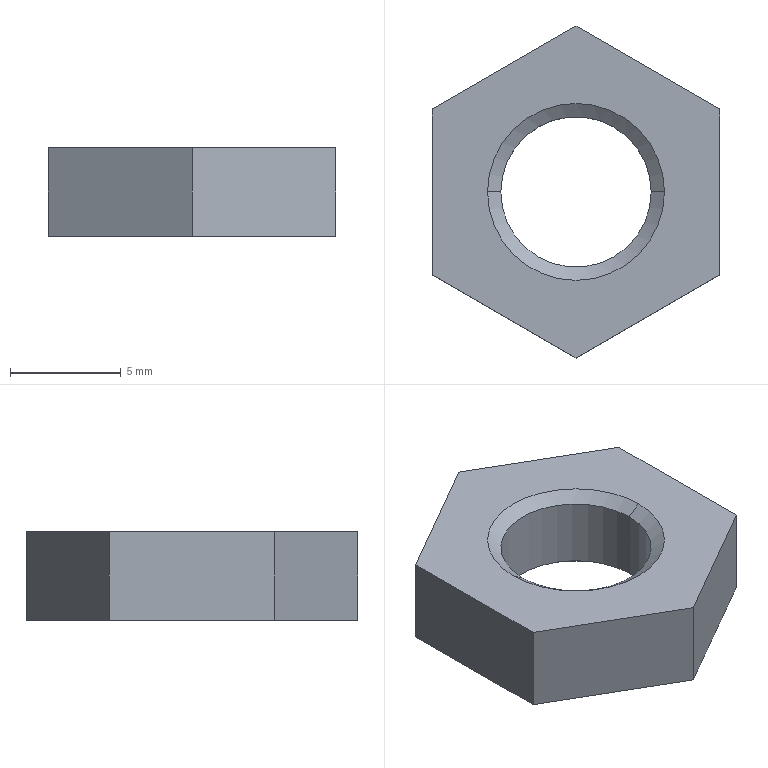Part | STEP file | hex thin nut gradeb_iso(Hexagon Nut ISO - 4036 - M8 - N) | 1 solid | 16 faces | box 13 x 15.011 x 4 mm | volume 434.11 mm3 | plane 8 | cylinder 4 | cone 4 | commonest cylinder face diameters 6.8 x2 8 x2
STEP:
#1=CARTESIAN_POINT('',(0.,0.,0.));
#2=DIRECTION('',(0.,0.,1.));
#3=DIRECTION('',(1.,0.,0.));
#4=AXIS2_PLACEMENT_3D('',#1,#2,#3);
#5=CARTESIAN_POINT('',(4.,0.,-4.));
#6=VERTEX_POINT('',#5);
#7=CARTESIAN_POINT('',(4.,0.,-3.975));
#8=VERTEX_POINT('',#7);
#9=CARTESIAN_POINT('',(4.,0.,-25.038));
#10=DIRECTION('',(0.,0.,1.));
#11=VECTOR('',#10,1.);
#12=LINE('',#9,#11);
#13=CARTESIAN_POINT('',(0.,0.,-25.038));
#14=DIRECTION('',(0.,0.,1.));
#15=DIRECTION('',(1.,0.,0.));
#16=AXIS2_PLACEMENT_3D('',#13,#14,#15);
#17=CYLINDRICAL_SURFACE('',#16,4.);
#18=CARTESIAN_POINT('',(6.283,0.));
#19=DIRECTION('',(0.,1.));
#20=VECTOR('',#19,1.);
#21=LINE('',#18,#20);
#22=(GEOMETRIC_REPRESENTATION_CONTEXT(2)PARAMETRIC_REPRESENTATION_CONTEXT()REPRESENTATION_CONTEXT('',''));
#23=DEFINITIONAL_REPRESENTATION('',(#21),#22);
#24=PCURVE('',#17,#23);
#25=CARTESIAN_POINT('',(0.,0.,-25.038));
#26=DIRECTION('',(0.,0.,1.));
#27=DIRECTION('',(1.,0.,0.));
#28=AXIS2_PLACEMENT_3D('',#25,#26,#27);
#29=CYLINDRICAL_SURFACE('',#28,4.);
#30=CARTESIAN_POINT('',(0.,0.));
#31=DIRECTION('',(0.,1.));
#32=VECTOR('',#31,1.);
#33=LINE('',#30,#32);
#34=(GEOMETRIC_REPRESENTATION_CONTEXT(2)PARAMETRIC_REPRESENTATION_CONTEXT()REPRESENTATION_CONTEXT('',''));
#35=DEFINITIONAL_REPRESENTATION('',(#33),#34);
#36=PCURVE('',#29,#35);
#37=SURFACE_CURVE('',#12,(#24,#36),.PCURVE_S1.);
#38=EDGE_CURVE('',#6,#8,#37,.T.);
#39=ORIENTED_EDGE('',*,*,#38,.T.);
#40=CARTESIAN_POINT('',(-4.,0.,-3.975));
#41=VERTEX_POINT('',#40);
#42=CARTESIAN_POINT('',(0.,0.,-3.975));
#43=DIRECTION('',(0.,0.,1.));
#44=DIRECTION('',(1.,0.,0.));
#45=AXIS2_PLACEMENT_3D('',#42,#43,#44);
#46=CIRCLE('',#45,4.);
#47=CARTESIAN_POINT('',(0.,21.063));
#48=DIRECTION('',(1.,0.));
#49=VECTOR('',#48,1.);
#50=LINE('',#47,#49);
#51=(GEOMETRIC_REPRESENTATION_CONTEXT(2)PARAMETRIC_REPRESENTATION_CONTEXT()REPRESENTATION_CONTEXT('',''));
#52=DEFINITIONAL_REPRESENTATION('',(#50),#51);
#53=PCURVE('',#17,#52);
#54=CARTESIAN_POINT('',(0.,0.,-3.975));
#55=DIRECTION('',(0.,0.,-1.));
#56=DIRECTION('',(-1.,0.,0.));
#57=AXIS2_PLACEMENT_3D('',#54,#55,#56);
#58=CONICAL_SURFACE('',#57,4.,0.9599);
#59=CARTESIAN_POINT('',(9.425,0.));
#60=DIRECTION('',(-1.,0.));
#61=VECTOR('',#60,1.);
#62=LINE('',#59,#61);
#63=(GEOMETRIC_REPRESENTATION_CONTEXT(2)PARAMETRIC_REPRESENTATION_CONTEXT()REPRESENTATION_CONTEXT('',''));
#64=DEFINITIONAL_REPRESENTATION('',(#62),#63);
#65=PCURVE('',#58,#64);
#66=SURFACE_CURVE('',#46,(#53,#65),.PCURVE_S1.);
#67=EDGE_CURVE('',#41,#8,#66,.T.);
#68=ORIENTED_EDGE('',*,*,#67,.F.);
#69=CARTESIAN_POINT('',(-4.,0.,-4.));
#70=VERTEX_POINT('',#69);
#71=CARTESIAN_POINT('',(-4.,0.,-25.038));
#72=DIRECTION('',(0.,0.,1.));
#73=VECTOR('',#72,1.);
#74=LINE('',#71,#73);
#75=CARTESIAN_POINT('',(3.142,0.));
#76=DIRECTION('',(0.,1.));
#77=VECTOR('',#76,1.);
#78=LINE('',#75,#77);
#79=(GEOMETRIC_REPRESENTATION_CONTEXT(2)PARAMETRIC_REPRESENTATION_CONTEXT()REPRESENTATION_CONTEXT('',''));
#80=DEFINITIONAL_REPRESENTATION('',(#78),#79);
#81=PCURVE('',#17,#80);
#82=CARTESIAN_POINT('',(3.142,0.));
#83=DIRECTION('',(0.,1.));
#84=VECTOR('',#83,1.);
#85=LINE('',#82,#84);
#86=(GEOMETRIC_REPRESENTATION_CONTEXT(2)PARAMETRIC_REPRESENTATION_CONTEXT()REPRESENTATION_CONTEXT('',''));
#87=DEFINITIONAL_REPRESENTATION('',(#85),#86);
#88=PCURVE('',#29,#87);
#89=SURFACE_CURVE('',#74,(#81,#88),.PCURVE_S1.);
#90=EDGE_CURVE('',#70,#41,#89,.T.);
#91=ORIENTED_EDGE('',*,*,#90,.F.);
#92=CARTESIAN_POINT('',(0.,0.,-4.));
#93=DIRECTION('',(0.,0.,1.));
#94=DIRECTION('',(-1.,0.,0.));
#95=AXIS2_PLACEMENT_3D('',#92,#93,#94);
#96=CIRCLE('',#95,4.);
#97=CARTESIAN_POINT('',(3.142,21.038));
#98=DIRECTION('',(1.,0.));
#99=VECTOR('',#98,1.);
#100=LINE('',#97,#99);
#101=(GEOMETRIC_REPRESENTATION_CONTEXT(2)PARAMETRIC_REPRESENTATION_CONTEXT()REPRESENTATION_CONTEXT('',''));
#102=DEFINITIONAL_REPRESENTATION('',(#100),#101);
#103=PCURVE('',#17,#102);
#104=CARTESIAN_POINT('',(0.,7.506,-4.));
#105=DIRECTION('',(0.,0.,-1.));
#106=DIRECTION('',(-1.,0.,0.));
#107=AXIS2_PLACEMENT_3D('',#104,#105,#106);
#108=PLANE('',#107);
#109=CARTESIAN_POINT('',(4.,-7.506));
#110=CARTESIAN_POINT('',(4.,-14.434));
#111=CARTESIAN_POINT('',(-2.,-10.97));
#112=CARTESIAN_POINT('',(-8.,-7.506));
#113=CARTESIAN_POINT('',(-2.,-4.041));
#114=CARTESIAN_POINT('',(4.,-0.5774));
#115=CARTESIAN_POINT('',(4.,-7.506));
#116=(BOUNDED_CURVE()B_SPLINE_CURVE(2,(#109,#110,#111,#112,#113,#114,#115),.UNSPECIFIED.,.T.,.F.)B_SPLINE_CURVE_WITH_KNOTS((1,2,2,2,2,1),(-2.094,0.,2.094,4.189,6.283,8.378),.UNSPECIFIED.)CURVE()GEOMETRIC_REPRESENTATION_ITEM()RATIONAL_B_SPLINE_CURVE((1.,0.5,1.,0.5,1.,0.5,1.))REPRESENTATION_ITEM(''));
#117=(GEOMETRIC_REPRESENTATION_CONTEXT(2)PARAMETRIC_REPRESENTATION_CONTEXT()REPRESENTATION_CONTEXT('',''));
#118=DEFINITIONAL_REPRESENTATION('',(#116),#117);
#119=PCURVE('',#108,#118);
#120=SURFACE_CURVE('',#96,(#103,#119),.PCURVE_S1.);
#121=EDGE_CURVE('',#70,#6,#120,.T.);
#122=ORIENTED_EDGE('',*,*,#121,.T.);
#123=EDGE_LOOP('',(#39,#68,#91,#122));
#124=FACE_BOUND('',#123,.F.);
#125=ADVANCED_FACE('',(#124),#17,.F.);
#126=CARTESIAN_POINT('',(-3.4,0.,-3.554));
#127=VERTEX_POINT('',#126);
#128=CARTESIAN_POINT('',(-4.,0.,-3.975));
#129=DIRECTION('',(-0.8192,0.,-0.5736));
#130=VECTOR('',#129,1.);
#131=LINE('',#128,#130);
#132=CARTESIAN_POINT('',(6.283,0.));
#133=DIRECTION('',(0.,1.));
#134=VECTOR('',#133,1.);
#135=LINE('',#132,#134);
#136=(GEOMETRIC_REPRESENTATION_CONTEXT(2)PARAMETRIC_REPRESENTATION_CONTEXT()REPRESENTATION_CONTEXT('',''));
#137=DEFINITIONAL_REPRESENTATION('',(#135),#136);
#138=PCURVE('',#58,#137);
#139=CARTESIAN_POINT('',(0.,0.,-3.975));
#140=DIRECTION('',(0.,0.,-1.));
#141=DIRECTION('',(-1.,0.,0.));
#142=AXIS2_PLACEMENT_3D('',#139,#140,#141);
#143=CONICAL_SURFACE('',#142,4.,0.9599);
#144=CARTESIAN_POINT('',(0.,0.));
#145=DIRECTION('',(0.,1.));
#146=VECTOR('',#145,1.);
#147=LINE('',#144,#146);
#148=(GEOMETRIC_REPRESENTATION_CONTEXT(2)PARAMETRIC_REPRESENTATION_CONTEXT()REPRESENTATION_CONTEXT('',''));
#149=DEFINITIONAL_REPRESENTATION('',(#147),#148);
#150=PCURVE('',#143,#149);
#151=SURFACE_CURVE('',#131,(#138,#150),.PCURVE_S1.);
#152=EDGE_CURVE('',#127,#41,#151,.T.);
#153=ORIENTED_EDGE('',*,*,#152,.T.);
#154=ORIENTED_EDGE('',*,*,#67,.T.);
#155=CARTESIAN_POINT('',(3.4,0.,-3.554));
#156=VERTEX_POINT('',#155);
#157=CARTESIAN_POINT('',(4.,0.,-3.975));
#158=DIRECTION('',(0.8192,0.,-0.5736));
#159=VECTOR('',#158,1.);
#160=LINE('',#157,#159);
#161=CARTESIAN_POINT('',(3.142,0.));
#162=DIRECTION('',(0.,1.));
#163=VECTOR('',#162,1.);
#164=LINE('',#161,#163);
#165=(GEOMETRIC_REPRESENTATION_CONTEXT(2)PARAMETRIC_REPRESENTATION_CONTEXT()REPRESENTATION_CONTEXT('',''));
#166=DEFINITIONAL_REPRESENTATION('',(#164),#165);
#167=PCURVE('',#58,#166);
#168=CARTESIAN_POINT('',(3.142,0.));
#169=DIRECTION('',(0.,1.));
#170=VECTOR('',#169,1.);
#171=LINE('',#168,#170);
#172=(GEOMETRIC_REPRESENTATION_CONTEXT(2)PARAMETRIC_REPRESENTATION_CONTEXT()REPRESENTATION_CONTEXT('',''));
#173=DEFINITIONAL_REPRESENTATION('',(#171),#172);
#174=PCURVE('',#143,#173);
#175=SURFACE_CURVE('',#160,(#167,#174),.PCURVE_S1.);
#176=EDGE_CURVE('',#156,#8,#175,.T.);
#177=ORIENTED_EDGE('',*,*,#176,.F.);
#178=CARTESIAN_POINT('',(0.,0.,-3.554));
#179=DIRECTION('',(0.,0.,1.));
#180=DIRECTION('',(-1.,0.,0.));
#181=AXIS2_PLACEMENT_3D('',#178,#179,#180);
#182=CIRCLE('',#181,3.4);
#183=CARTESIAN_POINT('',(6.283,-0.4201));
#184=DIRECTION('',(-1.,0.));
#185=VECTOR('',#184,1.);
#186=LINE('',#183,#185);
#187=(GEOMETRIC_REPRESENTATION_CONTEXT(2)PARAMETRIC_REPRESENTATION_CONTEXT()REPRESENTATION_CONTEXT('',''));
#188=DEFINITIONAL_REPRESENTATION('',(#186),#187);
#189=PCURVE('',#58,#188);
#190=CARTESIAN_POINT('',(0.,0.,-4.));
#191=DIRECTION('',(0.,0.,1.));
#192=DIRECTION('',(1.,0.,0.));
#193=AXIS2_PLACEMENT_3D('',#190,#191,#192);
#194=CYLINDRICAL_SURFACE('',#193,3.4);
#195=CARTESIAN_POINT('',(3.142,0.4455));
#196=DIRECTION('',(1.,0.));
#197=VECTOR('',#196,1.);
#198=LINE('',#195,#197);
#199=(GEOMETRIC_REPRESENTATION_CONTEXT(2)PARAMETRIC_REPRESENTATION_CONTEXT()REPRESENTATION_CONTEXT('',''));
#200=DEFINITIONAL_REPRESENTATION('',(#198),#199);
#201=PCURVE('',#194,#200);
#202=SURFACE_CURVE('',#182,(#189,#201),.PCURVE_S1.);
#203=EDGE_CURVE('',#127,#156,#202,.T.);
#204=ORIENTED_EDGE('',*,*,#203,.F.);
#205=EDGE_LOOP('',(#153,#154,#177,#204));
#206=FACE_BOUND('',#205,.F.);
#207=ADVANCED_FACE('',(#206),#58,.F.);
#208=CARTESIAN_POINT('',(3.4,0.,-0.4201));
#209=VERTEX_POINT('',#208);
#210=CARTESIAN_POINT('',(4.,0.,0.));
#211=VERTEX_POINT('',#210);
#212=CARTESIAN_POINT('',(3.34,0.,-0.4621));
#213=DIRECTION('',(0.8192,0.,0.5736));
#214=VECTOR('',#213,1.);
#215=LINE('',#212,#214);
#216=CARTESIAN_POINT('',(0.,0.,-0.4621));
#217=DIRECTION('',(0.,0.,1.));
#218=DIRECTION('',(1.,0.,0.));
#219=AXIS2_PLACEMENT_3D('',#216,#217,#218);
#220=CONICAL_SURFACE('',#219,3.34,0.9599);
#221=CARTESIAN_POINT('',(6.283,0.));
#222=DIRECTION('',(0.,1.));
#223=VECTOR('',#222,1.);
#224=LINE('',#221,#223);
#225=(GEOMETRIC_REPRESENTATION_CONTEXT(2)PARAMETRIC_REPRESENTATION_CONTEXT()REPRESENTATION_CONTEXT('',''));
#226=DEFINITIONAL_REPRESENTATION('',(#224),#225);
#227=PCURVE('',#220,#226);
#228=CARTESIAN_POINT('',(0.,0.,-0.4621));
#229=DIRECTION('',(0.,0.,1.));
#230=DIRECTION('',(1.,0.,0.));
#231=AXIS2_PLACEMENT_3D('',#228,#229,#230);
#232=CONICAL_SURFACE('',#231,3.34,0.9599);
#233=CARTESIAN_POINT('',(0.,0.));
#234=DIRECTION('',(0.,1.));
#235=VECTOR('',#234,1.);
#236=LINE('',#233,#235);
#237=(GEOMETRIC_REPRESENTATION_CONTEXT(2)PARAMETRIC_REPRESENTATION_CONTEXT()REPRESENTATION_CONTEXT('',''));
#238=DEFINITIONAL_REPRESENTATION('',(#236),#237);
#239=PCURVE('',#232,#238);
#240=SURFACE_CURVE('',#215,(#227,#239),.PCURVE_S1.);
#241=EDGE_CURVE('',#209,#211,#240,.T.);
#242=ORIENTED_EDGE('',*,*,#241,.T.);
#243=CARTESIAN_POINT('',(-4.,0.,0.));
#244=VERTEX_POINT('',#243);
#245=CARTESIAN_POINT('',(0.,0.,0.));
#246=DIRECTION('',(0.,0.,1.));
#247=DIRECTION('',(1.,0.,0.));
#248=AXIS2_PLACEMENT_3D('',#245,#246,#247);
#249=CIRCLE('',#248,4.);
#250=CARTESIAN_POINT('',(0.,0.4621));
#251=DIRECTION('',(1.,0.));
#252=VECTOR('',#251,1.);
#253=LINE('',#250,#252);
#254=(GEOMETRIC_REPRESENTATION_CONTEXT(2)PARAMETRIC_REPRESENTATION_CONTEXT()REPRESENTATION_CONTEXT('',''));
#255=DEFINITIONAL_REPRESENTATION('',(#253),#254);
#256=PCURVE('',#220,#255);
#257=CARTESIAN_POINT('',(0.,7.506,0.));
#258=DIRECTION('',(0.,0.,-1.));
#259=DIRECTION('',(-1.,0.,0.));
#260=AXIS2_PLACEMENT_3D('',#257,#258,#259);
#261=PLANE('',#260);
#262=CARTESIAN_POINT('',(-4.,-7.506));
#263=CARTESIAN_POINT('',(-4.,-0.5774));
#264=CARTESIAN_POINT('',(2.,-4.041));
#265=CARTESIAN_POINT('',(8.,-7.506));
#266=CARTESIAN_POINT('',(2.,-10.97));
#267=CARTESIAN_POINT('',(-4.,-14.434));
#268=CARTESIAN_POINT('',(-4.,-7.506));
#269=(BOUNDED_CURVE()B_SPLINE_CURVE(2,(#262,#263,#264,#265,#266,#267,#268),.UNSPECIFIED.,.T.,.F.)B_SPLINE_CURVE_WITH_KNOTS((1,2,2,2,2,1),(-2.094,0.,2.094,4.189,6.283,8.378),.UNSPECIFIED.)CURVE()GEOMETRIC_REPRESENTATION_ITEM()RATIONAL_B_SPLINE_CURVE((1.,0.5,1.,0.5,1.,0.5,1.))REPRESENTATION_ITEM(''));
#270=(GEOMETRIC_REPRESENTATION_CONTEXT(2)PARAMETRIC_REPRESENTATION_CONTEXT()REPRESENTATION_CONTEXT('',''));
#271=DEFINITIONAL_REPRESENTATION('',(#269),#270);
#272=PCURVE('',#261,#271);
#273=SURFACE_CURVE('',#249,(#256,#272),.PCURVE_S1.);
#274=EDGE_CURVE('',#244,#211,#273,.T.);
#275=ORIENTED_EDGE('',*,*,#274,.F.);
#276=CARTESIAN_POINT('',(-3.4,0.,-0.4201));
#277=VERTEX_POINT('',#276);
#278=CARTESIAN_POINT('',(-3.34,0.,-0.4621));
#279=DIRECTION('',(-0.8192,0.,0.5736));
#280=VECTOR('',#279,1.);
#281=LINE('',#278,#280);
#282=CARTESIAN_POINT('',(3.142,0.));
#283=DIRECTION('',(0.,1.));
#284=VECTOR('',#283,1.);
#285=LINE('',#282,#284);
#286=(GEOMETRIC_REPRESENTATION_CONTEXT(2)PARAMETRIC_REPRESENTATION_CONTEXT()REPRESENTATION_CONTEXT('',''));
#287=DEFINITIONAL_REPRESENTATION('',(#285),#286);
#288=PCURVE('',#220,#287);
#289=CARTESIAN_POINT('',(3.142,0.));
#290=DIRECTION('',(0.,1.));
#291=VECTOR('',#290,1.);
#292=LINE('',#289,#291);
#293=(GEOMETRIC_REPRESENTATION_CONTEXT(2)PARAMETRIC_REPRESENTATION_CONTEXT()REPRESENTATION_CONTEXT('',''));
#294=DEFINITIONAL_REPRESENTATION('',(#292),#293);
#295=PCURVE('',#232,#294);
#296=SURFACE_CURVE('',#281,(#288,#295),.PCURVE_S1.);
#297=EDGE_CURVE('',#277,#244,#296,.T.);
#298=ORIENTED_EDGE('',*,*,#297,.F.);
#299=CARTESIAN_POINT('',(0.,0.,-0.4201));
#300=DIRECTION('',(0.,0.,-1.));
#301=DIRECTION('',(1.,0.,0.));
#302=AXIS2_PLACEMENT_3D('',#299,#300,#301);
#303=CIRCLE('',#302,3.4);
#304=CARTESIAN_POINT('',(6.283,0.04201));
#305=DIRECTION('',(-1.,0.));
#306=VECTOR('',#305,1.);
#307=LINE('',#304,#306);
#308=(GEOMETRIC_REPRESENTATION_CONTEXT(2)PARAMETRIC_REPRESENTATION_CONTEXT()REPRESENTATION_CONTEXT('',''));
#309=DEFINITIONAL_REPRESENTATION('',(#307),#308);
#310=PCURVE('',#220,#309);
#311=CARTESIAN_POINT('',(6.283,3.58));
#312=DIRECTION('',(-1.,0.));
#313=VECTOR('',#312,1.);
#314=LINE('',#311,#313);
#315=(GEOMETRIC_REPRESENTATION_CONTEXT(2)PARAMETRIC_REPRESENTATION_CONTEXT()REPRESENTATION_CONTEXT('',''));
#316=DEFINITIONAL_REPRESENTATION('',(#314),#315);
#317=PCURVE('',#194,#316);
#318=SURFACE_CURVE('',#303,(#310,#317),.PCURVE_S1.);
#319=EDGE_CURVE('',#209,#277,#318,.T.);
#320=ORIENTED_EDGE('',*,*,#319,.F.);
#321=EDGE_LOOP('',(#242,#275,#298,#320));
#322=FACE_BOUND('',#321,.F.);
#323=ADVANCED_FACE('',(#322),#220,.F.);
#324=CARTESIAN_POINT('',(3.4,0.,-4.));
#325=DIRECTION('',(0.,0.,1.));
#326=VECTOR('',#325,1.);
#327=LINE('',#324,#326);
#328=CARTESIAN_POINT('',(6.283,0.));
#329=DIRECTION('',(0.,1.));
#330=VECTOR('',#329,1.);
#331=LINE('',#328,#330);
#332=(GEOMETRIC_REPRESENTATION_CONTEXT(2)PARAMETRIC_REPRESENTATION_CONTEXT()REPRESENTATION_CONTEXT('',''));
#333=DEFINITIONAL_REPRESENTATION('',(#331),#332);
#334=PCURVE('',#194,#333);
#335=CARTESIAN_POINT('',(0.,0.,-4.));
#336=DIRECTION('',(0.,0.,1.));
#337=DIRECTION('',(1.,0.,0.));
#338=AXIS2_PLACEMENT_3D('',#335,#336,#337);
#339=CYLINDRICAL_SURFACE('',#338,3.4);
#340=CARTESIAN_POINT('',(0.,0.));
#341=DIRECTION('',(0.,1.));
#342=VECTOR('',#341,1.);
#343=LINE('',#340,#342);
#344=(GEOMETRIC_REPRESENTATION_CONTEXT(2)PARAMETRIC_REPRESENTATION_CONTEXT()REPRESENTATION_CONTEXT('',''));
#345=DEFINITIONAL_REPRESENTATION('',(#343),#344);
#346=PCURVE('',#339,#345);
#347=SURFACE_CURVE('',#327,(#334,#346),.PCURVE_S1.);
#348=EDGE_CURVE('',#156,#209,#347,.T.);
#349=ORIENTED_EDGE('',*,*,#348,.T.);
#350=ORIENTED_EDGE('',*,*,#319,.T.);
#351=CARTESIAN_POINT('',(-3.4,0.,-4.));
#352=DIRECTION('',(0.,0.,1.));
#353=VECTOR('',#352,1.);
#354=LINE('',#351,#353);
#355=CARTESIAN_POINT('',(3.142,0.));
#356=DIRECTION('',(0.,1.));
#357=VECTOR('',#356,1.);
#358=LINE('',#355,#357);
#359=(GEOMETRIC_REPRESENTATION_CONTEXT(2)PARAMETRIC_REPRESENTATION_CONTEXT()REPRESENTATION_CONTEXT('',''));
#360=DEFINITIONAL_REPRESENTATION('',(#358),#359);
#361=PCURVE('',#194,#360);
#362=CARTESIAN_POINT('',(3.142,0.));
#363=DIRECTION('',(0.,1.));
#364=VECTOR('',#363,1.);
#365=LINE('',#362,#364);
#366=(GEOMETRIC_REPRESENTATION_CONTEXT(2)PARAMETRIC_REPRESENTATION_CONTEXT()REPRESENTATION_CONTEXT('',''));
#367=DEFINITIONAL_REPRESENTATION('',(#365),#366);
#368=PCURVE('',#339,#367);
#369=SURFACE_CURVE('',#354,(#361,#368),.PCURVE_S1.);
#370=EDGE_CURVE('',#127,#277,#369,.T.);
#371=ORIENTED_EDGE('',*,*,#370,.F.);
#372=ORIENTED_EDGE('',*,*,#203,.T.);
#373=EDGE_LOOP('',(#349,#350,#371,#372));
#374=FACE_BOUND('',#373,.F.);
#375=ADVANCED_FACE('',(#374),#194,.F.);
#376=CARTESIAN_POINT('',(0.,0.,-0.4201));
#377=DIRECTION('',(0.,0.,-1.));
#378=DIRECTION('',(1.,0.,0.));
#379=AXIS2_PLACEMENT_3D('',#376,#377,#378);
#380=CIRCLE('',#379,3.4);
#381=CARTESIAN_POINT('',(6.283,3.58));
#382=DIRECTION('',(-1.,0.));
#383=VECTOR('',#382,1.);
#384=LINE('',#381,#383);
#385=(GEOMETRIC_REPRESENTATION_CONTEXT(2)PARAMETRIC_REPRESENTATION_CONTEXT()REPRESENTATION_CONTEXT('',''));
#386=DEFINITIONAL_REPRESENTATION('',(#384),#385);
#387=PCURVE('',#339,#386);
#388=CARTESIAN_POINT('',(6.283,0.04201));
#389=DIRECTION('',(-1.,0.));
#390=VECTOR('',#389,1.);
#391=LINE('',#388,#390);
#392=(GEOMETRIC_REPRESENTATION_CONTEXT(2)PARAMETRIC_REPRESENTATION_CONTEXT()REPRESENTATION_CONTEXT('',''));
#393=DEFINITIONAL_REPRESENTATION('',(#391),#392);
#394=PCURVE('',#232,#393);
#395=SURFACE_CURVE('',#380,(#387,#394),.PCURVE_S1.);
#396=EDGE_CURVE('',#277,#209,#395,.T.);
#397=ORIENTED_EDGE('',*,*,#396,.T.);
#398=ORIENTED_EDGE('',*,*,#348,.F.);
#399=CARTESIAN_POINT('',(0.,0.,-3.554));
#400=DIRECTION('',(0.,0.,1.));
#401=DIRECTION('',(-1.,0.,0.));
#402=AXIS2_PLACEMENT_3D('',#399,#400,#401);
#403=CIRCLE('',#402,3.4);
#404=CARTESIAN_POINT('',(-3.142,0.4455));
#405=DIRECTION('',(1.,0.));
#406=VECTOR('',#405,1.);
#407=LINE('',#404,#406);
#408=(GEOMETRIC_REPRESENTATION_CONTEXT(2)PARAMETRIC_REPRESENTATION_CONTEXT()REPRESENTATION_CONTEXT('',''));
#409=DEFINITIONAL_REPRESENTATION('',(#407),#408);
#410=PCURVE('',#339,#409);
#411=CARTESIAN_POINT('',(6.283,-0.4201));
#412=DIRECTION('',(-1.,0.));
#413=VECTOR('',#412,1.);
#414=LINE('',#411,#413);
#415=(GEOMETRIC_REPRESENTATION_CONTEXT(2)PARAMETRIC_REPRESENTATION_CONTEXT()REPRESENTATION_CONTEXT('',''));
#416=DEFINITIONAL_REPRESENTATION('',(#414),#415);
#417=PCURVE('',#143,#416);
#418=SURFACE_CURVE('',#403,(#410,#417),.PCURVE_S1.);
#419=EDGE_CURVE('',#156,#127,#418,.T.);
#420=ORIENTED_EDGE('',*,*,#419,.T.);
#421=ORIENTED_EDGE('',*,*,#370,.T.);
#422=EDGE_LOOP('',(#397,#398,#420,#421));
#423=FACE_BOUND('',#422,.F.);
#424=ADVANCED_FACE('',(#423),#339,.F.);
#425=CARTESIAN_POINT('',(0.,7.506,-4.));
#426=VERTEX_POINT('',#425);
#427=CARTESIAN_POINT('',(-6.5,3.753,-4.));
#428=VERTEX_POINT('',#427);
#429=CARTESIAN_POINT('',(0.,7.506,-4.));
#430=DIRECTION('',(-0.866,-0.5,0.));
#431=VECTOR('',#430,1.);
#432=LINE('',#429,#431);
#433=CARTESIAN_POINT('',(0.,0.));
#434=DIRECTION('',(0.866,-0.5));
#435=VECTOR('',#434,1.);
#436=LINE('',#433,#435);
#437=(GEOMETRIC_REPRESENTATION_CONTEXT(2)PARAMETRIC_REPRESENTATION_CONTEXT()REPRESENTATION_CONTEXT('',''));
#438=DEFINITIONAL_REPRESENTATION('',(#436),#437);
#439=PCURVE('',#108,#438);
#440=CARTESIAN_POINT('',(0.,7.506,-4.));
#441=DIRECTION('',(-0.5,0.866,0.));
#442=DIRECTION('',(-0.866,-0.5,0.));
#443=AXIS2_PLACEMENT_3D('',#440,#441,#442);
#444=PLANE('',#443);
#445=CARTESIAN_POINT('',(0.,0.));
#446=DIRECTION('',(1.,0.));
#447=VECTOR('',#446,1.);
#448=LINE('',#445,#447);
#449=(GEOMETRIC_REPRESENTATION_CONTEXT(2)PARAMETRIC_REPRESENTATION_CONTEXT()REPRESENTATION_CONTEXT('',''));
#450=DEFINITIONAL_REPRESENTATION('',(#448),#449);
#451=PCURVE('',#444,#450);
#452=SURFACE_CURVE('',#432,(#439,#451),.PCURVE_S1.);
#453=EDGE_CURVE('',#426,#428,#452,.T.);
#454=ORIENTED_EDGE('',*,*,#453,.F.);
#455=CARTESIAN_POINT('',(6.5,3.753,-4.));
#456=VERTEX_POINT('',#455);
#457=CARTESIAN_POINT('',(6.5,3.753,-4.));
#458=DIRECTION('',(-0.866,0.5,0.));
#459=VECTOR('',#458,1.);
#460=LINE('',#457,#459);
#461=CARTESIAN_POINT('',(-6.5,-3.753));
#462=DIRECTION('',(0.866,0.5));
#463=VECTOR('',#462,1.);
#464=LINE('',#461,#463);
#465=(GEOMETRIC_REPRESENTATION_CONTEXT(2)PARAMETRIC_REPRESENTATION_CONTEXT()REPRESENTATION_CONTEXT('',''));
#466=DEFINITIONAL_REPRESENTATION('',(#464),#465);
#467=PCURVE('',#108,#466);
#468=CARTESIAN_POINT('',(6.5,3.753,-4.));
#469=DIRECTION('',(0.5,0.866,0.));
#470=DIRECTION('',(-0.866,0.5,0.));
#471=AXIS2_PLACEMENT_3D('',#468,#469,#470);
#472=PLANE('',#471);
#473=CARTESIAN_POINT('',(0.,0.));
#474=DIRECTION('',(1.,0.));
#475=VECTOR('',#474,1.);
#476=LINE('',#473,#475);
#477=(GEOMETRIC_REPRESENTATION_CONTEXT(2)PARAMETRIC_REPRESENTATION_CONTEXT()REPRESENTATION_CONTEXT('',''));
#478=DEFINITIONAL_REPRESENTATION('',(#476),#477);
#479=PCURVE('',#472,#478);
#480=SURFACE_CURVE('',#460,(#467,#479),.PCURVE_S1.);
#481=EDGE_CURVE('',#456,#426,#480,.T.);
#482=ORIENTED_EDGE('',*,*,#481,.F.);
#483=CARTESIAN_POINT('',(6.5,-3.753,-4.));
#484=VERTEX_POINT('',#483);
#485=CARTESIAN_POINT('',(6.5,3.753,-4.));
#486=DIRECTION('',(0.,-1.,0.));
#487=VECTOR('',#486,1.);
#488=LINE('',#485,#487);
#489=CARTESIAN_POINT('',(-6.5,-3.753));
#490=DIRECTION('',(0.,-1.));
#491=VECTOR('',#490,1.);
#492=LINE('',#489,#491);
#493=(GEOMETRIC_REPRESENTATION_CONTEXT(2)PARAMETRIC_REPRESENTATION_CONTEXT()REPRESENTATION_CONTEXT('',''));
#494=DEFINITIONAL_REPRESENTATION('',(#492),#493);
#495=PCURVE('',#108,#494);
#496=CARTESIAN_POINT('',(6.5,3.753,-4.));
#497=DIRECTION('',(-1.,0.,0.));
#498=DIRECTION('',(0.,0.,1.));
#499=AXIS2_PLACEMENT_3D('',#496,#497,#498);
#500=PLANE('',#499);
#501=CARTESIAN_POINT('',(0.,0.));
#502=DIRECTION('',(0.,-1.));
#503=VECTOR('',#502,1.);
#504=LINE('',#501,#503);
#505=(GEOMETRIC_REPRESENTATION_CONTEXT(2)PARAMETRIC_REPRESENTATION_CONTEXT()REPRESENTATION_CONTEXT('',''));
#506=DEFINITIONAL_REPRESENTATION('',(#504),#505);
#507=PCURVE('',#500,#506);
#508=SURFACE_CURVE('',#488,(#495,#507),.PCURVE_S1.);
#509=EDGE_CURVE('',#456,#484,#508,.T.);
#510=ORIENTED_EDGE('',*,*,#509,.T.);
#511=CARTESIAN_POINT('',(0.,-7.506,-4.));
#512=VERTEX_POINT('',#511);
#513=CARTESIAN_POINT('',(0.,-7.506,-4.));
#514=DIRECTION('',(0.866,0.5,0.));
#515=VECTOR('',#514,1.);
#516=LINE('',#513,#515);
#517=CARTESIAN_POINT('',(0.,-15.011));
#518=DIRECTION('',(-0.866,0.5));
#519=VECTOR('',#518,1.);
#520=LINE('',#517,#519);
#521=(GEOMETRIC_REPRESENTATION_CONTEXT(2)PARAMETRIC_REPRESENTATION_CONTEXT()REPRESENTATION_CONTEXT('',''));
#522=DEFINITIONAL_REPRESENTATION('',(#520),#521);
#523=PCURVE('',#108,#522);
#524=CARTESIAN_POINT('',(0.,-7.506,-4.));
#525=DIRECTION('',(0.5,-0.866,0.));
#526=DIRECTION('',(0.866,0.5,0.));
#527=AXIS2_PLACEMENT_3D('',#524,#525,#526);
#528=PLANE('',#527);
#529=CARTESIAN_POINT('',(0.,0.));
#530=DIRECTION('',(1.,0.));
#531=VECTOR('',#530,1.);
#532=LINE('',#529,#531);
#533=(GEOMETRIC_REPRESENTATION_CONTEXT(2)PARAMETRIC_REPRESENTATION_CONTEXT()REPRESENTATION_CONTEXT('',''));
#534=DEFINITIONAL_REPRESENTATION('',(#532),#533);
#535=PCURVE('',#528,#534);
#536=SURFACE_CURVE('',#516,(#523,#535),.PCURVE_S1.);
#537=EDGE_CURVE('',#512,#484,#536,.T.);
#538=ORIENTED_EDGE('',*,*,#537,.F.);
#539=CARTESIAN_POINT('',(-6.5,-3.753,-4.));
#540=VERTEX_POINT('',#539);
#541=CARTESIAN_POINT('',(-6.5,-3.753,-4.));
#542=DIRECTION('',(0.866,-0.5,0.));
#543=VECTOR('',#542,1.);
#544=LINE('',#541,#543);
#545=CARTESIAN_POINT('',(6.5,-11.258));
#546=DIRECTION('',(-0.866,-0.5));
#547=VECTOR('',#546,1.);
#548=LINE('',#545,#547);
#549=(GEOMETRIC_REPRESENTATION_CONTEXT(2)PARAMETRIC_REPRESENTATION_CONTEXT()REPRESENTATION_CONTEXT('',''));
#550=DEFINITIONAL_REPRESENTATION('',(#548),#549);
#551=PCURVE('',#108,#550);
#552=CARTESIAN_POINT('',(-6.5,-3.753,-4.));
#553=DIRECTION('',(-0.5,-0.866,0.));
#554=DIRECTION('',(0.866,-0.5,0.));
#555=AXIS2_PLACEMENT_3D('',#552,#553,#554);
#556=PLANE('',#555);
#557=CARTESIAN_POINT('',(0.,0.));
#558=DIRECTION('',(1.,0.));
#559=VECTOR('',#558,1.);
#560=LINE('',#557,#559);
#561=(GEOMETRIC_REPRESENTATION_CONTEXT(2)PARAMETRIC_REPRESENTATION_CONTEXT()REPRESENTATION_CONTEXT('',''));
#562=DEFINITIONAL_REPRESENTATION('',(#560),#561);
#563=PCURVE('',#556,#562);
#564=SURFACE_CURVE('',#544,(#551,#563),.PCURVE_S1.);
#565=EDGE_CURVE('',#540,#512,#564,.T.);
#566=ORIENTED_EDGE('',*,*,#565,.F.);
#567=CARTESIAN_POINT('',(-6.5,3.753,-4.));
#568=DIRECTION('',(0.,-1.,0.));
#569=VECTOR('',#568,1.);
#570=LINE('',#567,#569);
#571=CARTESIAN_POINT('',(6.5,-3.753));
#572=DIRECTION('',(0.,-1.));
#573=VECTOR('',#572,1.);
#574=LINE('',#571,#573);
#575=(GEOMETRIC_REPRESENTATION_CONTEXT(2)PARAMETRIC_REPRESENTATION_CONTEXT()REPRESENTATION_CONTEXT('',''));
#576=DEFINITIONAL_REPRESENTATION('',(#574),#575);
#577=PCURVE('',#108,#576);
#578=CARTESIAN_POINT('',(-6.5,3.753,-4.));
#579=DIRECTION('',(-1.,0.,0.));
#580=DIRECTION('',(0.,0.,1.));
#581=AXIS2_PLACEMENT_3D('',#578,#579,#580);
#582=PLANE('',#581);
#583=CARTESIAN_POINT('',(0.,0.));
#584=DIRECTION('',(0.,-1.));
#585=VECTOR('',#584,1.);
#586=LINE('',#583,#585);
#587=(GEOMETRIC_REPRESENTATION_CONTEXT(2)PARAMETRIC_REPRESENTATION_CONTEXT()REPRESENTATION_CONTEXT('',''));
#588=DEFINITIONAL_REPRESENTATION('',(#586),#587);
#589=PCURVE('',#582,#588);
#590=SURFACE_CURVE('',#570,(#577,#589),.PCURVE_S1.);
#591=EDGE_CURVE('',#428,#540,#590,.T.);
#592=ORIENTED_EDGE('',*,*,#591,.F.);
#593=EDGE_LOOP('',(#454,#482,#510,#538,#566,#592));
#594=FACE_BOUND('',#593,.T.);
#595=CARTESIAN_POINT('',(0.,0.,-4.));
#596=DIRECTION('',(0.,0.,1.));
#597=DIRECTION('',(-1.,0.,0.));
#598=AXIS2_PLACEMENT_3D('',#595,#596,#597);
#599=CIRCLE('',#598,4.);
#600=CARTESIAN_POINT('',(4.,-7.506));
#601=CARTESIAN_POINT('',(4.,-14.434));
#602=CARTESIAN_POINT('',(-2.,-10.97));
#603=CARTESIAN_POINT('',(-8.,-7.506));
#604=CARTESIAN_POINT('',(-2.,-4.041));
#605=CARTESIAN_POINT('',(4.,-0.5774));
#606=CARTESIAN_POINT('',(4.,-7.506));
#607=(BOUNDED_CURVE()B_SPLINE_CURVE(2,(#600,#601,#602,#603,#604,#605,#606),.UNSPECIFIED.,.T.,.F.)B_SPLINE_CURVE_WITH_KNOTS((1,2,2,2,2,1),(-2.094,0.,2.094,4.189,6.283,8.378),.UNSPECIFIED.)CURVE()GEOMETRIC_REPRESENTATION_ITEM()RATIONAL_B_SPLINE_CURVE((1.,0.5,1.,0.5,1.,0.5,1.))REPRESENTATION_ITEM(''));
#608=(GEOMETRIC_REPRESENTATION_CONTEXT(2)PARAMETRIC_REPRESENTATION_CONTEXT()REPRESENTATION_CONTEXT('',''));
#609=DEFINITIONAL_REPRESENTATION('',(#607),#608);
#610=PCURVE('',#108,#609);
#611=CARTESIAN_POINT('',(-3.142,21.038));
#612=DIRECTION('',(1.,0.));
#613=VECTOR('',#612,1.);
#614=LINE('',#611,#613);
#615=(GEOMETRIC_REPRESENTATION_CONTEXT(2)PARAMETRIC_REPRESENTATION_CONTEXT()REPRESENTATION_CONTEXT('',''));
#616=DEFINITIONAL_REPRESENTATION('',(#614),#615);
#617=PCURVE('',#29,#616);
#618=SURFACE_CURVE('',#599,(#610,#617),.PCURVE_S1.);
#619=EDGE_CURVE('',#6,#70,#618,.T.);
#620=ORIENTED_EDGE('',*,*,#619,.T.);
#621=ORIENTED_EDGE('',*,*,#121,.T.);
#622=EDGE_LOOP('',(#620,#621));
#623=FACE_BOUND('',#622,.T.);
#624=ADVANCED_FACE('',(#594,#623),#108,.T.);
#625=CARTESIAN_POINT('',(0.,7.506,0.));
#626=VERTEX_POINT('',#625);
#627=CARTESIAN_POINT('',(-6.5,3.753,0.));
#628=VERTEX_POINT('',#627);
#629=CARTESIAN_POINT('',(0.,7.506,0.));
#630=DIRECTION('',(-0.866,-0.5,0.));
#631=VECTOR('',#630,1.);
#632=LINE('',#629,#631);
#633=CARTESIAN_POINT('',(0.,0.));
#634=DIRECTION('',(0.866,-0.5));
#635=VECTOR('',#634,1.);
#636=LINE('',#633,#635);
#637=(GEOMETRIC_REPRESENTATION_CONTEXT(2)PARAMETRIC_REPRESENTATION_CONTEXT()REPRESENTATION_CONTEXT('',''));
#638=DEFINITIONAL_REPRESENTATION('',(#636),#637);
#639=PCURVE('',#261,#638);
#640=CARTESIAN_POINT('',(0.,4.));
#641=DIRECTION('',(1.,0.));
#642=VECTOR('',#641,1.);
#643=LINE('',#640,#642);
#644=(GEOMETRIC_REPRESENTATION_CONTEXT(2)PARAMETRIC_REPRESENTATION_CONTEXT()REPRESENTATION_CONTEXT('',''));
#645=DEFINITIONAL_REPRESENTATION('',(#643),#644);
#646=PCURVE('',#444,#645);
#647=SURFACE_CURVE('',#632,(#639,#646),.PCURVE_S1.);
#648=EDGE_CURVE('',#626,#628,#647,.T.);
#649=ORIENTED_EDGE('',*,*,#648,.T.);
#650=CARTESIAN_POINT('',(-6.5,-3.753,0.));
#651=VERTEX_POINT('',#650);
#652=CARTESIAN_POINT('',(-6.5,3.753,0.));
#653=DIRECTION('',(0.,-1.,0.));
#654=VECTOR('',#653,1.);
#655=LINE('',#652,#654);
#656=CARTESIAN_POINT('',(6.5,-3.753));
#657=DIRECTION('',(0.,-1.));
#658=VECTOR('',#657,1.);
#659=LINE('',#656,#658);
#660=(GEOMETRIC_REPRESENTATION_CONTEXT(2)PARAMETRIC_REPRESENTATION_CONTEXT()REPRESENTATION_CONTEXT('',''));
#661=DEFINITIONAL_REPRESENTATION('',(#659),#660);
#662=PCURVE('',#261,#661);
#663=CARTESIAN_POINT('',(4.,0.));
#664=DIRECTION('',(0.,-1.));
#665=VECTOR('',#664,1.);
#666=LINE('',#663,#665);
#667=(GEOMETRIC_REPRESENTATION_CONTEXT(2)PARAMETRIC_REPRESENTATION_CONTEXT()REPRESENTATION_CONTEXT('',''));
#668=DEFINITIONAL_REPRESENTATION('',(#666),#667);
#669=PCURVE('',#582,#668);
#670=SURFACE_CURVE('',#655,(#662,#669),.PCURVE_S1.);
#671=EDGE_CURVE('',#628,#651,#670,.T.);
#672=ORIENTED_EDGE('',*,*,#671,.T.);
#673=CARTESIAN_POINT('',(0.,-7.506,0.));
#674=VERTEX_POINT('',#673);
#675=CARTESIAN_POINT('',(-6.5,-3.753,0.));
#676=DIRECTION('',(0.866,-0.5,0.));
#677=VECTOR('',#676,1.);
#678=LINE('',#675,#677);
#679=CARTESIAN_POINT('',(6.5,-11.258));
#680=DIRECTION('',(-0.866,-0.5));
#681=VECTOR('',#680,1.);
#682=LINE('',#679,#681);
#683=(GEOMETRIC_REPRESENTATION_CONTEXT(2)PARAMETRIC_REPRESENTATION_CONTEXT()REPRESENTATION_CONTEXT('',''));
#684=DEFINITIONAL_REPRESENTATION('',(#682),#683);
#685=PCURVE('',#261,#684);
#686=CARTESIAN_POINT('',(0.,4.));
#687=DIRECTION('',(1.,0.));
#688=VECTOR('',#687,1.);
#689=LINE('',#686,#688);
#690=(GEOMETRIC_REPRESENTATION_CONTEXT(2)PARAMETRIC_REPRESENTATION_CONTEXT()REPRESENTATION_CONTEXT('',''));
#691=DEFINITIONAL_REPRESENTATION('',(#689),#690);
#692=PCURVE('',#556,#691);
#693=SURFACE_CURVE('',#678,(#685,#692),.PCURVE_S1.);
#694=EDGE_CURVE('',#651,#674,#693,.T.);
#695=ORIENTED_EDGE('',*,*,#694,.T.);
#696=CARTESIAN_POINT('',(6.5,-3.753,0.));
#697=VERTEX_POINT('',#696);
#698=CARTESIAN_POINT('',(0.,-7.506,0.));
#699=DIRECTION('',(0.866,0.5,0.));
#700=VECTOR('',#699,1.);
#701=LINE('',#698,#700);
#702=CARTESIAN_POINT('',(0.,-15.011));
#703=DIRECTION('',(-0.866,0.5));
#704=VECTOR('',#703,1.);
#705=LINE('',#702,#704);
#706=(GEOMETRIC_REPRESENTATION_CONTEXT(2)PARAMETRIC_REPRESENTATION_CONTEXT()REPRESENTATION_CONTEXT('',''));
#707=DEFINITIONAL_REPRESENTATION('',(#705),#706);
#708=PCURVE('',#261,#707);
#709=CARTESIAN_POINT('',(0.,4.));
#710=DIRECTION('',(1.,0.));
#711=VECTOR('',#710,1.);
#712=LINE('',#709,#711);
#713=(GEOMETRIC_REPRESENTATION_CONTEXT(2)PARAMETRIC_REPRESENTATION_CONTEXT()REPRESENTATION_CONTEXT('',''));
#714=DEFINITIONAL_REPRESENTATION('',(#712),#713);
#715=PCURVE('',#528,#714);
#716=SURFACE_CURVE('',#701,(#708,#715),.PCURVE_S1.);
#717=EDGE_CURVE('',#674,#697,#716,.T.);
#718=ORIENTED_EDGE('',*,*,#717,.T.);
#719=CARTESIAN_POINT('',(6.5,3.753,0.));
#720=VERTEX_POINT('',#719);
#721=CARTESIAN_POINT('',(6.5,3.753,0.));
#722=DIRECTION('',(0.,-1.,0.));
#723=VECTOR('',#722,1.);
#724=LINE('',#721,#723);
#725=CARTESIAN_POINT('',(-6.5,-3.753));
#726=DIRECTION('',(0.,-1.));
#727=VECTOR('',#726,1.);
#728=LINE('',#725,#727);
#729=(GEOMETRIC_REPRESENTATION_CONTEXT(2)PARAMETRIC_REPRESENTATION_CONTEXT()REPRESENTATION_CONTEXT('',''));
#730=DEFINITIONAL_REPRESENTATION('',(#728),#729);
#731=PCURVE('',#261,#730);
#732=CARTESIAN_POINT('',(4.,0.));
#733=DIRECTION('',(0.,-1.));
#734=VECTOR('',#733,1.);
#735=LINE('',#732,#734);
#736=(GEOMETRIC_REPRESENTATION_CONTEXT(2)PARAMETRIC_REPRESENTATION_CONTEXT()REPRESENTATION_CONTEXT('',''));
#737=DEFINITIONAL_REPRESENTATION('',(#735),#736);
#738=PCURVE('',#500,#737);
#739=SURFACE_CURVE('',#724,(#731,#738),.PCURVE_S1.);
#740=EDGE_CURVE('',#720,#697,#739,.T.);
#741=ORIENTED_EDGE('',*,*,#740,.F.);
#742=CARTESIAN_POINT('',(6.5,3.753,0.));
#743=DIRECTION('',(-0.866,0.5,0.));
#744=VECTOR('',#743,1.);
#745=LINE('',#742,#744);
#746=CARTESIAN_POINT('',(-6.5,-3.753));
#747=DIRECTION('',(0.866,0.5));
#748=VECTOR('',#747,1.);
#749=LINE('',#746,#748);
#750=(GEOMETRIC_REPRESENTATION_CONTEXT(2)PARAMETRIC_REPRESENTATION_CONTEXT()REPRESENTATION_CONTEXT('',''));
#751=DEFINITIONAL_REPRESENTATION('',(#749),#750);
#752=PCURVE('',#261,#751);
#753=CARTESIAN_POINT('',(0.,4.));
#754=DIRECTION('',(1.,0.));
#755=VECTOR('',#754,1.);
#756=LINE('',#753,#755);
#757=(GEOMETRIC_REPRESENTATION_CONTEXT(2)PARAMETRIC_REPRESENTATION_CONTEXT()REPRESENTATION_CONTEXT('',''));
#758=DEFINITIONAL_REPRESENTATION('',(#756),#757);
#759=PCURVE('',#472,#758);
#760=SURFACE_CURVE('',#745,(#752,#759),.PCURVE_S1.);
#761=EDGE_CURVE('',#720,#626,#760,.T.);
#762=ORIENTED_EDGE('',*,*,#761,.T.);
#763=EDGE_LOOP('',(#649,#672,#695,#718,#741,#762));
#764=FACE_BOUND('',#763,.T.);
#765=CARTESIAN_POINT('',(0.,0.,0.));
#766=DIRECTION('',(0.,0.,1.));
#767=DIRECTION('',(1.,0.,0.));
#768=AXIS2_PLACEMENT_3D('',#765,#766,#767);
#769=CIRCLE('',#768,4.);
#770=CARTESIAN_POINT('',(-4.,-7.506));
#771=CARTESIAN_POINT('',(-4.,-0.5774));
#772=CARTESIAN_POINT('',(2.,-4.041));
#773=CARTESIAN_POINT('',(8.,-7.506));
#774=CARTESIAN_POINT('',(2.,-10.97));
#775=CARTESIAN_POINT('',(-4.,-14.434));
#776=CARTESIAN_POINT('',(-4.,-7.506));
#777=(BOUNDED_CURVE()B_SPLINE_CURVE(2,(#770,#771,#772,#773,#774,#775,#776),.UNSPECIFIED.,.T.,.F.)B_SPLINE_CURVE_WITH_KNOTS((1,2,2,2,2,1),(-2.094,0.,2.094,4.189,6.283,8.378),.UNSPECIFIED.)CURVE()GEOMETRIC_REPRESENTATION_ITEM()RATIONAL_B_SPLINE_CURVE((1.,0.5,1.,0.5,1.,0.5,1.))REPRESENTATION_ITEM(''));
#778=(GEOMETRIC_REPRESENTATION_CONTEXT(2)PARAMETRIC_REPRESENTATION_CONTEXT()REPRESENTATION_CONTEXT('',''));
#779=DEFINITIONAL_REPRESENTATION('',(#777),#778);
#780=PCURVE('',#261,#779);
#781=CARTESIAN_POINT('',(0.,0.4621));
#782=DIRECTION('',(1.,0.));
#783=VECTOR('',#782,1.);
#784=LINE('',#781,#783);
#785=(GEOMETRIC_REPRESENTATION_CONTEXT(2)PARAMETRIC_REPRESENTATION_CONTEXT()REPRESENTATION_CONTEXT('',''));
#786=DEFINITIONAL_REPRESENTATION('',(#784),#785);
#787=PCURVE('',#232,#786);
#788=SURFACE_CURVE('',#769,(#780,#787),.PCURVE_S1.);
#789=EDGE_CURVE('',#211,#244,#788,.T.);
#790=ORIENTED_EDGE('',*,*,#789,.F.);
#791=ORIENTED_EDGE('',*,*,#274,.F.);
#792=EDGE_LOOP('',(#790,#791));
#793=FACE_BOUND('',#792,.T.);
#794=ADVANCED_FACE('',(#764,#793),#261,.F.);
#795=ORIENTED_EDGE('',*,*,#648,.F.);
#796=CARTESIAN_POINT('',(0.,7.506,-4.));
#797=DIRECTION('',(0.,0.,1.));
#798=VECTOR('',#797,1.);
#799=LINE('',#796,#798);
#800=CARTESIAN_POINT('',(0.,0.));
#801=DIRECTION('',(0.,1.));
#802=VECTOR('',#801,1.);
#803=LINE('',#800,#802);
#804=(GEOMETRIC_REPRESENTATION_CONTEXT(2)PARAMETRIC_REPRESENTATION_CONTEXT()REPRESENTATION_CONTEXT('',''));
#805=DEFINITIONAL_REPRESENTATION('',(#803),#804);
#806=PCURVE('',#444,#805);
#807=CARTESIAN_POINT('',(7.506,0.));
#808=DIRECTION('',(0.,1.));
#809=VECTOR('',#808,1.);
#810=LINE('',#807,#809);
#811=(GEOMETRIC_REPRESENTATION_CONTEXT(2)PARAMETRIC_REPRESENTATION_CONTEXT()REPRESENTATION_CONTEXT('',''));
#812=DEFINITIONAL_REPRESENTATION('',(#810),#811);
#813=PCURVE('',#472,#812);
#814=SURFACE_CURVE('',#799,(#806,#813),.PCURVE_S1.);
#815=EDGE_CURVE('',#426,#626,#814,.T.);
#816=ORIENTED_EDGE('',*,*,#815,.F.);
#817=ORIENTED_EDGE('',*,*,#453,.T.);
#818=CARTESIAN_POINT('',(-6.5,3.753,-4.));
#819=DIRECTION('',(0.,0.,1.));
#820=VECTOR('',#819,1.);
#821=LINE('',#818,#820);
#822=CARTESIAN_POINT('',(7.506,0.));
#823=DIRECTION('',(0.,1.));
#824=VECTOR('',#823,1.);
#825=LINE('',#822,#824);
#826=(GEOMETRIC_REPRESENTATION_CONTEXT(2)PARAMETRIC_REPRESENTATION_CONTEXT()REPRESENTATION_CONTEXT('',''));
#827=DEFINITIONAL_REPRESENTATION('',(#825),#826);
#828=PCURVE('',#444,#827);
#829=CARTESIAN_POINT('',(0.,0.));
#830=DIRECTION('',(1.,0.));
#831=VECTOR('',#830,1.);
#832=LINE('',#829,#831);
#833=(GEOMETRIC_REPRESENTATION_CONTEXT(2)PARAMETRIC_REPRESENTATION_CONTEXT()REPRESENTATION_CONTEXT('',''));
#834=DEFINITIONAL_REPRESENTATION('',(#832),#833);
#835=PCURVE('',#582,#834);
#836=SURFACE_CURVE('',#821,(#828,#835),.PCURVE_S1.);
#837=EDGE_CURVE('',#428,#628,#836,.T.);
#838=ORIENTED_EDGE('',*,*,#837,.T.);
#839=EDGE_LOOP('',(#795,#816,#817,#838));
#840=FACE_BOUND('',#839,.T.);
#841=ADVANCED_FACE('',(#840),#444,.T.);
#842=ORIENTED_EDGE('',*,*,#761,.F.);
#843=CARTESIAN_POINT('',(6.5,3.753,-4.));
#844=DIRECTION('',(0.,0.,1.));
#845=VECTOR('',#844,1.);
#846=LINE('',#843,#845);
#847=CARTESIAN_POINT('',(0.,0.));
#848=DIRECTION('',(0.,1.));
#849=VECTOR('',#848,1.);
#850=LINE('',#847,#849);
#851=(GEOMETRIC_REPRESENTATION_CONTEXT(2)PARAMETRIC_REPRESENTATION_CONTEXT()REPRESENTATION_CONTEXT('',''));
#852=DEFINITIONAL_REPRESENTATION('',(#850),#851);
#853=PCURVE('',#472,#852);
#854=CARTESIAN_POINT('',(0.,0.));
#855=DIRECTION('',(1.,0.));
#856=VECTOR('',#855,1.);
#857=LINE('',#854,#856);
#858=(GEOMETRIC_REPRESENTATION_CONTEXT(2)PARAMETRIC_REPRESENTATION_CONTEXT()REPRESENTATION_CONTEXT('',''));
#859=DEFINITIONAL_REPRESENTATION('',(#857),#858);
#860=PCURVE('',#500,#859);
#861=SURFACE_CURVE('',#846,(#853,#860),.PCURVE_S1.);
#862=EDGE_CURVE('',#456,#720,#861,.T.);
#863=ORIENTED_EDGE('',*,*,#862,.F.);
#864=ORIENTED_EDGE('',*,*,#481,.T.);
#865=ORIENTED_EDGE('',*,*,#815,.T.);
#866=EDGE_LOOP('',(#842,#863,#864,#865));
#867=FACE_BOUND('',#866,.T.);
#868=ADVANCED_FACE('',(#867),#472,.T.);
#869=ORIENTED_EDGE('',*,*,#740,.T.);
#870=CARTESIAN_POINT('',(6.5,-3.753,-4.));
#871=DIRECTION('',(0.,0.,1.));
#872=VECTOR('',#871,1.);
#873=LINE('',#870,#872);
#874=CARTESIAN_POINT('',(0.,-7.506));
#875=DIRECTION('',(1.,0.));
#876=VECTOR('',#875,1.);
#877=LINE('',#874,#876);
#878=(GEOMETRIC_REPRESENTATION_CONTEXT(2)PARAMETRIC_REPRESENTATION_CONTEXT()REPRESENTATION_CONTEXT('',''));
#879=DEFINITIONAL_REPRESENTATION('',(#877),#878);
#880=PCURVE('',#500,#879);
#881=CARTESIAN_POINT('',(7.506,0.));
#882=DIRECTION('',(0.,1.));
#883=VECTOR('',#882,1.);
#884=LINE('',#881,#883);
#885=(GEOMETRIC_REPRESENTATION_CONTEXT(2)PARAMETRIC_REPRESENTATION_CONTEXT()REPRESENTATION_CONTEXT('',''));
#886=DEFINITIONAL_REPRESENTATION('',(#884),#885);
#887=PCURVE('',#528,#886);
#888=SURFACE_CURVE('',#873,(#880,#887),.PCURVE_S1.);
#889=EDGE_CURVE('',#484,#697,#888,.T.);
#890=ORIENTED_EDGE('',*,*,#889,.F.);
#891=ORIENTED_EDGE('',*,*,#509,.F.);
#892=ORIENTED_EDGE('',*,*,#862,.T.);
#893=EDGE_LOOP('',(#869,#890,#891,#892));
#894=FACE_BOUND('',#893,.T.);
#895=ADVANCED_FACE('',(#894),#500,.F.);
#896=ORIENTED_EDGE('',*,*,#717,.F.);
#897=CARTESIAN_POINT('',(0.,-7.506,-4.));
#898=DIRECTION('',(0.,0.,1.));
#899=VECTOR('',#898,1.);
#900=LINE('',#897,#899);
#901=CARTESIAN_POINT('',(0.,0.));
#902=DIRECTION('',(0.,1.));
#903=VECTOR('',#902,1.);
#904=LINE('',#901,#903);
#905=(GEOMETRIC_REPRESENTATION_CONTEXT(2)PARAMETRIC_REPRESENTATION_CONTEXT()REPRESENTATION_CONTEXT('',''));
#906=DEFINITIONAL_REPRESENTATION('',(#904),#905);
#907=PCURVE('',#528,#906);
#908=CARTESIAN_POINT('',(7.506,0.));
#909=DIRECTION('',(0.,1.));
#910=VECTOR('',#909,1.);
#911=LINE('',#908,#910);
#912=(GEOMETRIC_REPRESENTATION_CONTEXT(2)PARAMETRIC_REPRESENTATION_CONTEXT()REPRESENTATION_CONTEXT('',''));
#913=DEFINITIONAL_REPRESENTATION('',(#911),#912);
#914=PCURVE('',#556,#913);
#915=SURFACE_CURVE('',#900,(#907,#914),.PCURVE_S1.);
#916=EDGE_CURVE('',#512,#674,#915,.T.);
#917=ORIENTED_EDGE('',*,*,#916,.F.);
#918=ORIENTED_EDGE('',*,*,#537,.T.);
#919=ORIENTED_EDGE('',*,*,#889,.T.);
#920=EDGE_LOOP('',(#896,#917,#918,#919));
#921=FACE_BOUND('',#920,.T.);
#922=ADVANCED_FACE('',(#921),#528,.T.);
#923=ORIENTED_EDGE('',*,*,#694,.F.);
#924=CARTESIAN_POINT('',(-6.5,-3.753,-4.));
#925=DIRECTION('',(0.,0.,1.));
#926=VECTOR('',#925,1.);
#927=LINE('',#924,#926);
#928=CARTESIAN_POINT('',(0.,0.));
#929=DIRECTION('',(0.,1.));
#930=VECTOR('',#929,1.);
#931=LINE('',#928,#930);
#932=(GEOMETRIC_REPRESENTATION_CONTEXT(2)PARAMETRIC_REPRESENTATION_CONTEXT()REPRESENTATION_CONTEXT('',''));
#933=DEFINITIONAL_REPRESENTATION('',(#931),#932);
#934=PCURVE('',#556,#933);
#935=CARTESIAN_POINT('',(0.,-7.506));
#936=DIRECTION('',(1.,0.));
#937=VECTOR('',#936,1.);
#938=LINE('',#935,#937);
#939=(GEOMETRIC_REPRESENTATION_CONTEXT(2)PARAMETRIC_REPRESENTATION_CONTEXT()REPRESENTATION_CONTEXT('',''));
#940=DEFINITIONAL_REPRESENTATION('',(#938),#939);
#941=PCURVE('',#582,#940);
#942=SURFACE_CURVE('',#927,(#934,#941),.PCURVE_S1.);
#943=EDGE_CURVE('',#540,#651,#942,.T.);
#944=ORIENTED_EDGE('',*,*,#943,.F.);
#945=ORIENTED_EDGE('',*,*,#565,.T.);
#946=ORIENTED_EDGE('',*,*,#916,.T.);
#947=EDGE_LOOP('',(#923,#944,#945,#946));
#948=FACE_BOUND('',#947,.T.);
#949=ADVANCED_FACE('',(#948),#556,.T.);
#950=ORIENTED_EDGE('',*,*,#671,.F.);
#951=ORIENTED_EDGE('',*,*,#837,.F.);
#952=ORIENTED_EDGE('',*,*,#591,.T.);
#953=ORIENTED_EDGE('',*,*,#943,.T.);
#954=EDGE_LOOP('',(#950,#951,#952,#953));
#955=FACE_BOUND('',#954,.T.);
#956=ADVANCED_FACE('',(#955),#582,.T.);
#957=ORIENTED_EDGE('',*,*,#789,.F.);
#958=ORIENTED_EDGE('',*,*,#241,.F.);
#959=ORIENTED_EDGE('',*,*,#396,.F.);
#960=ORIENTED_EDGE('',*,*,#297,.T.);
#961=EDGE_LOOP('',(#957,#958,#959,#960));
#962=FACE_BOUND('',#961,.F.);
#963=ADVANCED_FACE('',(#962),#232,.F.);
#964=CARTESIAN_POINT('',(0.,0.,-3.975));
#965=DIRECTION('',(0.,0.,1.));
#966=DIRECTION('',(1.,0.,0.));
#967=AXIS2_PLACEMENT_3D('',#964,#965,#966);
#968=CIRCLE('',#967,4.);
#969=CARTESIAN_POINT('',(3.142,0.));
#970=DIRECTION('',(-1.,0.));
#971=VECTOR('',#970,1.);
#972=LINE('',#969,#971);
#973=(GEOMETRIC_REPRESENTATION_CONTEXT(2)PARAMETRIC_REPRESENTATION_CONTEXT()REPRESENTATION_CONTEXT('',''));
#974=DEFINITIONAL_REPRESENTATION('',(#972),#973);
#975=PCURVE('',#143,#974);
#976=CARTESIAN_POINT('',(0.,21.063));
#977=DIRECTION('',(1.,0.));
#978=VECTOR('',#977,1.);
#979=LINE('',#976,#978);
#980=(GEOMETRIC_REPRESENTATION_CONTEXT(2)PARAMETRIC_REPRESENTATION_CONTEXT()REPRESENTATION_CONTEXT('',''));
#981=DEFINITIONAL_REPRESENTATION('',(#979),#980);
#982=PCURVE('',#29,#981);
#983=SURFACE_CURVE('',#968,(#975,#982),.PCURVE_S1.);
#984=EDGE_CURVE('',#8,#41,#983,.T.);
#985=ORIENTED_EDGE('',*,*,#984,.T.);
#986=ORIENTED_EDGE('',*,*,#152,.F.);
#987=ORIENTED_EDGE('',*,*,#419,.F.);
#988=ORIENTED_EDGE('',*,*,#176,.T.);
#989=EDGE_LOOP('',(#985,#986,#987,#988));
#990=FACE_BOUND('',#989,.F.);
#991=ADVANCED_FACE('',(#990),#143,.F.);
#992=ORIENTED_EDGE('',*,*,#984,.F.);
#993=ORIENTED_EDGE('',*,*,#38,.F.);
#994=ORIENTED_EDGE('',*,*,#619,.T.);
#995=ORIENTED_EDGE('',*,*,#90,.T.);
#996=EDGE_LOOP('',(#992,#993,#994,#995));
#997=FACE_BOUND('',#996,.F.);
#998=ADVANCED_FACE('',(#997),#29,.F.);
#999=CLOSED_SHELL('',(#125,#207,#323,#375,#424,#624,#794,#841,#868,#895,#922,#949,#956,#963,#991,#998));
#1000=MANIFOLD_SOLID_BREP('',#999);
#1001=(LENGTH_UNIT()NAMED_UNIT(*)SI_UNIT(.MILLI.,.METRE.));
#1002=UNCERTAINTY_MEASURE_WITH_UNIT(LENGTH_MEASURE(0.0000001),#1001,'','');
#1003=(NAMED_UNIT(*)PLANE_ANGLE_UNIT()SI_UNIT($,.RADIAN.));
#1004=(NAMED_UNIT(*)SI_UNIT($,.STERADIAN.)SOLID_ANGLE_UNIT());
#1005=(GEOMETRIC_REPRESENTATION_CONTEXT(3)GLOBAL_UNCERTAINTY_ASSIGNED_CONTEXT((#1002))GLOBAL_UNIT_ASSIGNED_CONTEXT((#1001,#1003,#1004))REPRESENTATION_CONTEXT('',''));
#1006=ADVANCED_BREP_SHAPE_REPRESENTATION('',(#4,#1000),#1005);